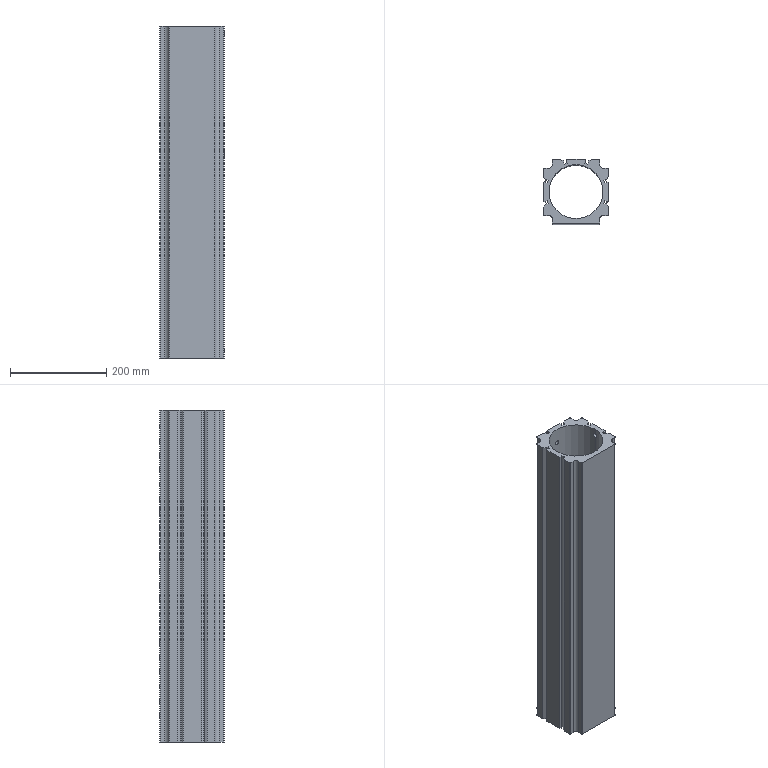Part | SolidWorks | features ICE 6, HoleWzd 5, Chamfer 3, CirPattern 3, Fillet 3, LPattern 2, MirrorPattern 2, Extrusion 1, MoveFace 1 | 1 solid | 136 faces | box 134 x 134 x 689 mm | volume 4449218 mm3 | plane 74 | cylinder 62 | commonest cylinder face diameters 9 x42 4 x8 8.8 x6 16 x4 112 x2